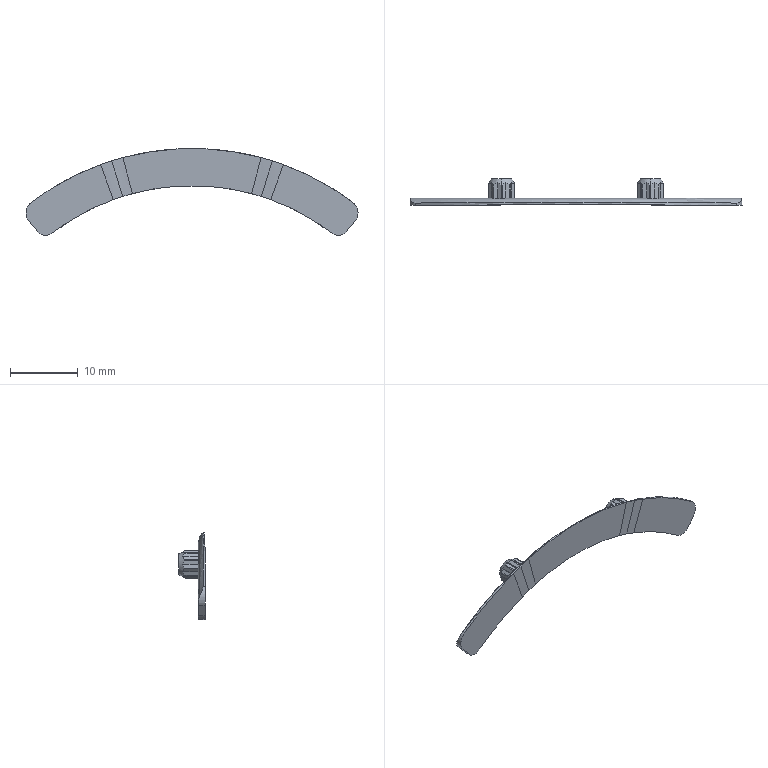Part | NX | features BREP 1 | 1 solid | 113 faces | box 49.082 x 3.9 x 12.866 mm | volume 307.576 mm3 | plane 48 | cylinder 46 | torus 9 | spline 6 | cone 4 | commonest cylinder face diameters 0.3 x40 3 x2 4 x2 68 x1 79 x1